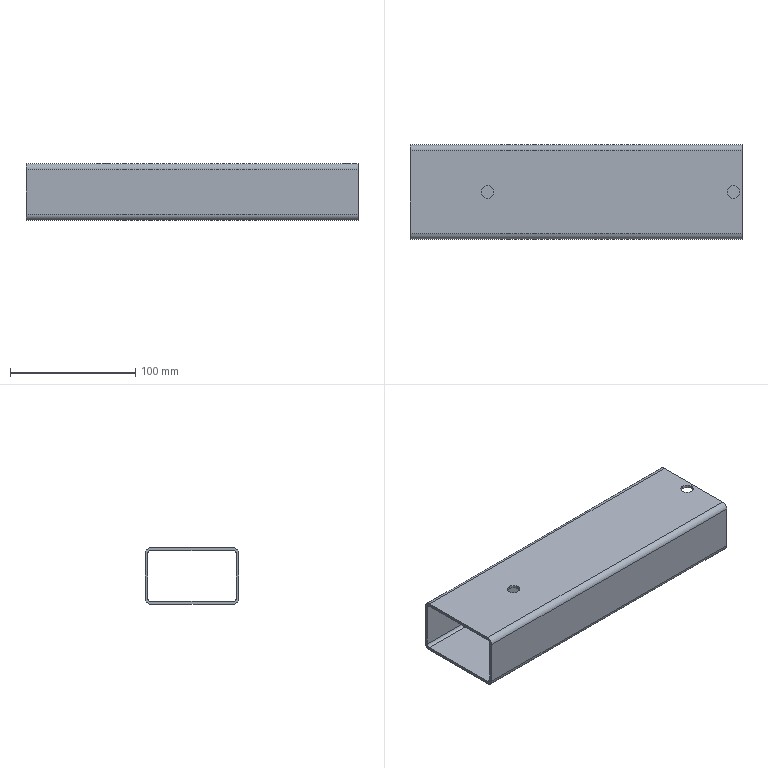Part | STEP file | [04]-1 | 1 solid | 22 faces | box 265 x 75 x 45 mm | volume 136701 mm3 | cylinder 12 | plane 10 | commonest cylinder face diameters 4.6 x4 9.2 x4 10 x4
STEP:
#1=CARTESIAN_POINT('',(81.9,42.5,45.));
#2=VERTEX_POINT('',#1);
#3=CARTESIAN_POINT('',(81.9,32.5,45.));
#4=VERTEX_POINT('',#3);
#5=CARTESIAN_POINT('',(81.9,37.5,45.));
#6=DIRECTION('',(0.,0.,-1.));
#7=DIRECTION('',(0.,-1.,0.));
#8=AXIS2_PLACEMENT_3D('',#5,#6,#7);
#9=CIRCLE('',#8,5.);
#10=EDGE_CURVE('',#2,#4,#9,.T.);
#11=ORIENTED_EDGE('',*,*,#10,.F.);
#12=CARTESIAN_POINT('',(81.9,42.5,42.7));
#13=VERTEX_POINT('',#12);
#14=CARTESIAN_POINT('',(81.9,42.5,45.));
#15=DIRECTION('',(0.,0.,-1.));
#16=VECTOR('',#15,1000.);
#17=LINE('',#14,#16);
#18=EDGE_CURVE('',#2,#13,#17,.T.);
#19=ORIENTED_EDGE('',*,*,#18,.T.);
#20=CARTESIAN_POINT('',(81.9,32.5,42.7));
#21=VERTEX_POINT('',#20);
#22=CARTESIAN_POINT('',(81.9,37.5,42.7));
#23=DIRECTION('',(0.,0.,1.));
#24=DIRECTION('',(0.,1.,0.));
#25=AXIS2_PLACEMENT_3D('',#22,#23,#24);
#26=CIRCLE('',#25,5.);
#27=EDGE_CURVE('',#21,#13,#26,.T.);
#28=ORIENTED_EDGE('',*,*,#27,.F.);
#29=CARTESIAN_POINT('',(81.9,32.5,45.));
#30=DIRECTION('',(0.,0.,-1.));
#31=VECTOR('',#30,1000.);
#32=LINE('',#29,#31);
#33=EDGE_CURVE('',#4,#21,#32,.T.);
#34=ORIENTED_EDGE('',*,*,#33,.F.);
#35=EDGE_LOOP('',(#11,#19,#28,#34));
#36=FACE_OUTER_BOUND('',#35,.T.);
#37=CARTESIAN_POINT('',(81.9,37.5,45.));
#38=DIRECTION('',(0.,0.,-1.));
#39=DIRECTION('',(0.,-1.,0.));
#40=AXIS2_PLACEMENT_3D('',#37,#38,#39);
#41=CYLINDRICAL_SURFACE('',#40,5.);
#42=ADVANCED_FACE('',(#36),#41,.F.);
#43=CARTESIAN_POINT('',(278.,42.5,45.));
#44=VERTEX_POINT('',#43);
#45=CARTESIAN_POINT('',(278.,32.5,45.));
#46=VERTEX_POINT('',#45);
#47=CARTESIAN_POINT('',(278.,37.5,45.));
#48=DIRECTION('',(0.,0.,-1.));
#49=DIRECTION('',(0.,-1.,0.));
#50=AXIS2_PLACEMENT_3D('',#47,#48,#49);
#51=CIRCLE('',#50,5.);
#52=EDGE_CURVE('',#44,#46,#51,.T.);
#53=ORIENTED_EDGE('',*,*,#52,.F.);
#54=CARTESIAN_POINT('',(278.,42.5,42.7));
#55=VERTEX_POINT('',#54);
#56=CARTESIAN_POINT('',(278.,42.5,45.));
#57=DIRECTION('',(0.,0.,-1.));
#58=VECTOR('',#57,1000.);
#59=LINE('',#56,#58);
#60=EDGE_CURVE('',#44,#55,#59,.T.);
#61=ORIENTED_EDGE('',*,*,#60,.T.);
#62=CARTESIAN_POINT('',(278.,32.5,42.7));
#63=VERTEX_POINT('',#62);
#64=CARTESIAN_POINT('',(278.,37.5,42.7));
#65=DIRECTION('',(0.,0.,1.));
#66=DIRECTION('',(0.,1.,0.));
#67=AXIS2_PLACEMENT_3D('',#64,#65,#66);
#68=CIRCLE('',#67,5.);
#69=EDGE_CURVE('',#63,#55,#68,.T.);
#70=ORIENTED_EDGE('',*,*,#69,.F.);
#71=CARTESIAN_POINT('',(278.,32.5,45.));
#72=DIRECTION('',(0.,0.,-1.));
#73=VECTOR('',#72,1000.);
#74=LINE('',#71,#73);
#75=EDGE_CURVE('',#46,#63,#74,.T.);
#76=ORIENTED_EDGE('',*,*,#75,.F.);
#77=EDGE_LOOP('',(#53,#61,#70,#76));
#78=FACE_OUTER_BOUND('',#77,.T.);
#79=CARTESIAN_POINT('',(278.,37.5,45.));
#80=DIRECTION('',(0.,0.,-1.));
#81=DIRECTION('',(0.,-1.,0.));
#82=AXIS2_PLACEMENT_3D('',#79,#80,#81);
#83=CYLINDRICAL_SURFACE('',#82,5.);
#84=ADVANCED_FACE('',(#78),#83,.F.);
#85=CARTESIAN_POINT('',(20.,70.4,0.));
#86=VERTEX_POINT('',#85);
#87=CARTESIAN_POINT('',(20.,4.6,0.));
#88=VERTEX_POINT('',#87);
#89=CARTESIAN_POINT('',(20.,70.4,0.));
#90=DIRECTION('',(0.,-1.,0.));
#91=VECTOR('',#90,1000.);
#92=LINE('',#89,#91);
#93=EDGE_CURVE('',#86,#88,#92,.T.);
#94=ORIENTED_EDGE('',*,*,#93,.T.);
#95=CARTESIAN_POINT('',(20.,0.,4.6));
#96=VERTEX_POINT('',#95);
#97=CARTESIAN_POINT('',(20.,4.6,4.6));
#98=DIRECTION('',(-1.,0.,0.));
#99=DIRECTION('',(0.,0.,-1.));
#100=AXIS2_PLACEMENT_3D('',#97,#98,#99);
#101=CIRCLE('',#100,4.6);
#102=EDGE_CURVE('',#88,#96,#101,.T.);
#103=ORIENTED_EDGE('',*,*,#102,.T.);
#104=CARTESIAN_POINT('',(20.,0.,40.4));
#105=VERTEX_POINT('',#104);
#106=CARTESIAN_POINT('',(20.,0.,4.6));
#107=DIRECTION('',(0.,0.,1.));
#108=VECTOR('',#107,1000.);
#109=LINE('',#106,#108);
#110=EDGE_CURVE('',#96,#105,#109,.T.);
#111=ORIENTED_EDGE('',*,*,#110,.T.);
#112=CARTESIAN_POINT('',(20.,4.6,45.));
#113=VERTEX_POINT('',#112);
#114=CARTESIAN_POINT('',(20.,4.6,40.4));
#115=DIRECTION('',(-1.,0.,0.));
#116=DIRECTION('',(0.,0.,-1.));
#117=AXIS2_PLACEMENT_3D('',#114,#115,#116);
#118=CIRCLE('',#117,4.6);
#119=EDGE_CURVE('',#105,#113,#118,.T.);
#120=ORIENTED_EDGE('',*,*,#119,.T.);
#121=CARTESIAN_POINT('',(20.,70.4,45.));
#122=VERTEX_POINT('',#121);
#123=CARTESIAN_POINT('',(20.,4.6,45.));
#124=DIRECTION('',(0.,1.,0.));
#125=VECTOR('',#124,1000.);
#126=LINE('',#123,#125);
#127=EDGE_CURVE('',#113,#122,#126,.T.);
#128=ORIENTED_EDGE('',*,*,#127,.T.);
#129=CARTESIAN_POINT('',(20.,75.,40.4));
#130=VERTEX_POINT('',#129);
#131=CARTESIAN_POINT('',(20.,70.4,40.4));
#132=DIRECTION('',(-1.,0.,0.));
#133=DIRECTION('',(0.,0.,-1.));
#134=AXIS2_PLACEMENT_3D('',#131,#132,#133);
#135=CIRCLE('',#134,4.6);
#136=EDGE_CURVE('',#122,#130,#135,.T.);
#137=ORIENTED_EDGE('',*,*,#136,.T.);
#138=CARTESIAN_POINT('',(20.,75.,4.6));
#139=VERTEX_POINT('',#138);
#140=CARTESIAN_POINT('',(20.,75.,40.4));
#141=DIRECTION('',(0.,0.,-1.));
#142=VECTOR('',#141,1000.);
#143=LINE('',#140,#142);
#144=EDGE_CURVE('',#130,#139,#143,.T.);
#145=ORIENTED_EDGE('',*,*,#144,.T.);
#146=CARTESIAN_POINT('',(20.,70.4,4.6));
#147=DIRECTION('',(-1.,0.,0.));
#148=DIRECTION('',(0.,0.,-1.));
#149=AXIS2_PLACEMENT_3D('',#146,#147,#148);
#150=CIRCLE('',#149,4.6);
#151=EDGE_CURVE('',#139,#86,#150,.T.);
#152=ORIENTED_EDGE('',*,*,#151,.T.);
#153=EDGE_LOOP('',(#94,#103,#111,#120,#128,#137,#145,#152));
#154=FACE_OUTER_BOUND('',#153,.T.);
#155=CARTESIAN_POINT('',(20.,70.4,2.3));
#156=VERTEX_POINT('',#155);
#157=CARTESIAN_POINT('',(20.,4.6,2.3));
#158=VERTEX_POINT('',#157);
#159=CARTESIAN_POINT('',(20.,70.4,2.3));
#160=DIRECTION('',(0.,-1.,0.));
#161=VECTOR('',#160,1000.);
#162=LINE('',#159,#161);
#163=EDGE_CURVE('',#156,#158,#162,.T.);
#164=ORIENTED_EDGE('',*,*,#163,.F.);
#165=CARTESIAN_POINT('',(20.,72.7,4.6));
#166=VERTEX_POINT('',#165);
#167=CARTESIAN_POINT('',(20.,70.4,4.6));
#168=DIRECTION('',(-1.,0.,0.));
#169=DIRECTION('',(0.,1.,0.));
#170=AXIS2_PLACEMENT_3D('',#167,#168,#169);
#171=CIRCLE('',#170,2.3);
#172=EDGE_CURVE('',#166,#156,#171,.T.);
#173=ORIENTED_EDGE('',*,*,#172,.F.);
#174=CARTESIAN_POINT('',(20.,72.7,40.4));
#175=VERTEX_POINT('',#174);
#176=CARTESIAN_POINT('',(20.,72.7,40.4));
#177=DIRECTION('',(0.,0.,-1.));
#178=VECTOR('',#177,1000.);
#179=LINE('',#176,#178);
#180=EDGE_CURVE('',#175,#166,#179,.T.);
#181=ORIENTED_EDGE('',*,*,#180,.F.);
#182=CARTESIAN_POINT('',(20.,70.4,42.7));
#183=VERTEX_POINT('',#182);
#184=CARTESIAN_POINT('',(20.,70.4,40.4));
#185=DIRECTION('',(-1.,0.,0.));
#186=DIRECTION('',(0.,1.,0.));
#187=AXIS2_PLACEMENT_3D('',#184,#185,#186);
#188=CIRCLE('',#187,2.3);
#189=EDGE_CURVE('',#183,#175,#188,.T.);
#190=ORIENTED_EDGE('',*,*,#189,.F.);
#191=CARTESIAN_POINT('',(20.,4.6,42.7));
#192=VERTEX_POINT('',#191);
#193=CARTESIAN_POINT('',(20.,4.6,42.7));
#194=DIRECTION('',(0.,1.,0.));
#195=VECTOR('',#194,1000.);
#196=LINE('',#193,#195);
#197=EDGE_CURVE('',#192,#183,#196,.T.);
#198=ORIENTED_EDGE('',*,*,#197,.F.);
#199=CARTESIAN_POINT('',(20.,2.3,40.4));
#200=VERTEX_POINT('',#199);
#201=CARTESIAN_POINT('',(20.,4.6,40.4));
#202=DIRECTION('',(-1.,0.,0.));
#203=DIRECTION('',(0.,1.,0.));
#204=AXIS2_PLACEMENT_3D('',#201,#202,#203);
#205=CIRCLE('',#204,2.3);
#206=EDGE_CURVE('',#200,#192,#205,.T.);
#207=ORIENTED_EDGE('',*,*,#206,.F.);
#208=CARTESIAN_POINT('',(20.,2.3,4.6));
#209=VERTEX_POINT('',#208);
#210=CARTESIAN_POINT('',(20.,2.3,4.6));
#211=DIRECTION('',(0.,0.,1.));
#212=VECTOR('',#211,1000.);
#213=LINE('',#210,#212);
#214=EDGE_CURVE('',#209,#200,#213,.T.);
#215=ORIENTED_EDGE('',*,*,#214,.F.);
#216=CARTESIAN_POINT('',(20.,4.6,4.6));
#217=DIRECTION('',(-1.,0.,0.));
#218=DIRECTION('',(0.,1.,0.));
#219=AXIS2_PLACEMENT_3D('',#216,#217,#218);
#220=CIRCLE('',#219,2.3);
#221=EDGE_CURVE('',#158,#209,#220,.T.);
#222=ORIENTED_EDGE('',*,*,#221,.F.);
#223=EDGE_LOOP('',(#164,#173,#181,#190,#198,#207,#215,#222));
#224=FACE_BOUND('',#223,.T.);
#225=CARTESIAN_POINT('',(20.,4.6,4.6));
#226=DIRECTION('',(-1.,0.,0.));
#227=DIRECTION('',(0.,0.,-1.));
#228=AXIS2_PLACEMENT_3D('',#225,#226,#227);
#229=PLANE('',#228);
#230=ADVANCED_FACE('',(#154,#224),#229,.T.);
#231=CARTESIAN_POINT('',(285.,70.4,0.));
#232=VERTEX_POINT('',#231);
#233=CARTESIAN_POINT('',(285.,4.6,0.));
#234=VERTEX_POINT('',#233);
#235=CARTESIAN_POINT('',(285.,70.4,0.));
#236=DIRECTION('',(0.,-1.,0.));
#237=VECTOR('',#236,1000.);
#238=LINE('',#235,#237);
#239=EDGE_CURVE('',#232,#234,#238,.T.);
#240=ORIENTED_EDGE('',*,*,#239,.F.);
#241=CARTESIAN_POINT('',(285.,75.,4.6));
#242=VERTEX_POINT('',#241);
#243=CARTESIAN_POINT('',(285.,70.4,4.6));
#244=DIRECTION('',(-1.,0.,0.));
#245=DIRECTION('',(0.,0.,-1.));
#246=AXIS2_PLACEMENT_3D('',#243,#244,#245);
#247=CIRCLE('',#246,4.6);
#248=EDGE_CURVE('',#242,#232,#247,.T.);
#249=ORIENTED_EDGE('',*,*,#248,.F.);
#250=CARTESIAN_POINT('',(285.,75.,40.4));
#251=VERTEX_POINT('',#250);
#252=CARTESIAN_POINT('',(285.,75.,40.4));
#253=DIRECTION('',(0.,0.,-1.));
#254=VECTOR('',#253,1000.);
#255=LINE('',#252,#254);
#256=EDGE_CURVE('',#251,#242,#255,.T.);
#257=ORIENTED_EDGE('',*,*,#256,.F.);
#258=CARTESIAN_POINT('',(285.,70.4,45.));
#259=VERTEX_POINT('',#258);
#260=CARTESIAN_POINT('',(285.,70.4,40.4));
#261=DIRECTION('',(-1.,0.,0.));
#262=DIRECTION('',(0.,0.,-1.));
#263=AXIS2_PLACEMENT_3D('',#260,#261,#262);
#264=CIRCLE('',#263,4.6);
#265=EDGE_CURVE('',#259,#251,#264,.T.);
#266=ORIENTED_EDGE('',*,*,#265,.F.);
#267=CARTESIAN_POINT('',(285.,4.6,45.));
#268=VERTEX_POINT('',#267);
#269=CARTESIAN_POINT('',(285.,4.6,45.));
#270=DIRECTION('',(0.,1.,0.));
#271=VECTOR('',#270,1000.);
#272=LINE('',#269,#271);
#273=EDGE_CURVE('',#268,#259,#272,.T.);
#274=ORIENTED_EDGE('',*,*,#273,.F.);
#275=CARTESIAN_POINT('',(285.,0.,40.4));
#276=VERTEX_POINT('',#275);
#277=CARTESIAN_POINT('',(285.,4.6,40.4));
#278=DIRECTION('',(-1.,0.,0.));
#279=DIRECTION('',(0.,0.,-1.));
#280=AXIS2_PLACEMENT_3D('',#277,#278,#279);
#281=CIRCLE('',#280,4.6);
#282=EDGE_CURVE('',#276,#268,#281,.T.);
#283=ORIENTED_EDGE('',*,*,#282,.F.);
#284=CARTESIAN_POINT('',(285.,0.,4.6));
#285=VERTEX_POINT('',#284);
#286=CARTESIAN_POINT('',(285.,0.,4.6));
#287=DIRECTION('',(0.,0.,1.));
#288=VECTOR('',#287,1000.);
#289=LINE('',#286,#288);
#290=EDGE_CURVE('',#285,#276,#289,.T.);
#291=ORIENTED_EDGE('',*,*,#290,.F.);
#292=CARTESIAN_POINT('',(285.,4.6,4.6));
#293=DIRECTION('',(-1.,0.,0.));
#294=DIRECTION('',(0.,0.,-1.));
#295=AXIS2_PLACEMENT_3D('',#292,#293,#294);
#296=CIRCLE('',#295,4.6);
#297=EDGE_CURVE('',#234,#285,#296,.T.);
#298=ORIENTED_EDGE('',*,*,#297,.F.);
#299=EDGE_LOOP('',(#240,#249,#257,#266,#274,#283,#291,#298));
#300=FACE_OUTER_BOUND('',#299,.T.);
#301=CARTESIAN_POINT('',(285.,72.7,4.6));
#302=VERTEX_POINT('',#301);
#303=CARTESIAN_POINT('',(285.,70.4,2.3));
#304=VERTEX_POINT('',#303);
#305=CARTESIAN_POINT('',(285.,70.4,4.6));
#306=DIRECTION('',(-1.,0.,0.));
#307=DIRECTION('',(0.,1.,0.));
#308=AXIS2_PLACEMENT_3D('',#305,#306,#307);
#309=CIRCLE('',#308,2.3);
#310=EDGE_CURVE('',#302,#304,#309,.T.);
#311=ORIENTED_EDGE('',*,*,#310,.T.);
#312=CARTESIAN_POINT('',(285.,4.6,2.3));
#313=VERTEX_POINT('',#312);
#314=CARTESIAN_POINT('',(285.,70.4,2.3));
#315=DIRECTION('',(0.,-1.,0.));
#316=VECTOR('',#315,1000.);
#317=LINE('',#314,#316);
#318=EDGE_CURVE('',#304,#313,#317,.T.);
#319=ORIENTED_EDGE('',*,*,#318,.T.);
#320=CARTESIAN_POINT('',(285.,2.3,4.6));
#321=VERTEX_POINT('',#320);
#322=CARTESIAN_POINT('',(285.,4.6,4.6));
#323=DIRECTION('',(-1.,0.,0.));
#324=DIRECTION('',(0.,1.,0.));
#325=AXIS2_PLACEMENT_3D('',#322,#323,#324);
#326=CIRCLE('',#325,2.3);
#327=EDGE_CURVE('',#313,#321,#326,.T.);
#328=ORIENTED_EDGE('',*,*,#327,.T.);
#329=CARTESIAN_POINT('',(285.,2.3,40.4));
#330=VERTEX_POINT('',#329);
#331=CARTESIAN_POINT('',(285.,2.3,4.6));
#332=DIRECTION('',(0.,0.,1.));
#333=VECTOR('',#332,1000.);
#334=LINE('',#331,#333);
#335=EDGE_CURVE('',#321,#330,#334,.T.);
#336=ORIENTED_EDGE('',*,*,#335,.T.);
#337=CARTESIAN_POINT('',(285.,4.6,42.7));
#338=VERTEX_POINT('',#337);
#339=CARTESIAN_POINT('',(285.,4.6,40.4));
#340=DIRECTION('',(-1.,0.,0.));
#341=DIRECTION('',(0.,1.,0.));
#342=AXIS2_PLACEMENT_3D('',#339,#340,#341);
#343=CIRCLE('',#342,2.3);
#344=EDGE_CURVE('',#330,#338,#343,.T.);
#345=ORIENTED_EDGE('',*,*,#344,.T.);
#346=CARTESIAN_POINT('',(285.,70.4,42.7));
#347=VERTEX_POINT('',#346);
#348=CARTESIAN_POINT('',(285.,4.6,42.7));
#349=DIRECTION('',(0.,1.,0.));
#350=VECTOR('',#349,1000.);
#351=LINE('',#348,#350);
#352=EDGE_CURVE('',#338,#347,#351,.T.);
#353=ORIENTED_EDGE('',*,*,#352,.T.);
#354=CARTESIAN_POINT('',(285.,72.7,40.4));
#355=VERTEX_POINT('',#354);
#356=CARTESIAN_POINT('',(285.,70.4,40.4));
#357=DIRECTION('',(-1.,0.,0.));
#358=DIRECTION('',(0.,1.,0.));
#359=AXIS2_PLACEMENT_3D('',#356,#357,#358);
#360=CIRCLE('',#359,2.3);
#361=EDGE_CURVE('',#347,#355,#360,.T.);
#362=ORIENTED_EDGE('',*,*,#361,.T.);
#363=CARTESIAN_POINT('',(285.,72.7,40.4));
#364=DIRECTION('',(0.,0.,-1.));
#365=VECTOR('',#364,1000.);
#366=LINE('',#363,#365);
#367=EDGE_CURVE('',#355,#302,#366,.T.);
#368=ORIENTED_EDGE('',*,*,#367,.T.);
#369=EDGE_LOOP('',(#311,#319,#328,#336,#345,#353,#362,#368));
#370=FACE_BOUND('',#369,.T.);
#371=CARTESIAN_POINT('',(285.,4.6,4.6));
#372=DIRECTION('',(-1.,0.,0.));
#373=DIRECTION('',(0.,0.,-1.));
#374=AXIS2_PLACEMENT_3D('',#371,#372,#373);
#375=PLANE('',#374);
#376=ADVANCED_FACE('',(#300,#370),#375,.F.);
#377=ORIENTED_EDGE('',*,*,#239,.T.);
#378=CARTESIAN_POINT('',(20.,4.6,0.));
#379=DIRECTION('',(1.,0.,0.));
#380=VECTOR('',#379,1000.);
#381=LINE('',#378,#380);
#382=EDGE_CURVE('',#88,#234,#381,.T.);
#383=ORIENTED_EDGE('',*,*,#382,.F.);
#384=ORIENTED_EDGE('',*,*,#93,.F.);
#385=CARTESIAN_POINT('',(20.,70.4,0.));
#386=DIRECTION('',(1.,0.,0.));
#387=VECTOR('',#386,1000.);
#388=LINE('',#385,#387);
#389=EDGE_CURVE('',#86,#232,#388,.T.);
#390=ORIENTED_EDGE('',*,*,#389,.T.);
#391=EDGE_LOOP('',(#377,#383,#384,#390));
#392=FACE_OUTER_BOUND('',#391,.T.);
#393=CARTESIAN_POINT('',(20.,70.4,0.));
#394=DIRECTION('',(0.,0.,1.));
#395=DIRECTION('',(0.,1.,0.));
#396=AXIS2_PLACEMENT_3D('',#393,#394,#395);
#397=PLANE('',#396);
#398=ADVANCED_FACE('',(#392),#397,.F.);
#399=ORIENTED_EDGE('',*,*,#297,.T.);
#400=CARTESIAN_POINT('',(20.,0.,4.6));
#401=DIRECTION('',(1.,0.,0.));
#402=VECTOR('',#401,1000.);
#403=LINE('',#400,#402);
#404=EDGE_CURVE('',#96,#285,#403,.T.);
#405=ORIENTED_EDGE('',*,*,#404,.F.);
#406=ORIENTED_EDGE('',*,*,#102,.F.);
#407=ORIENTED_EDGE('',*,*,#382,.T.);
#408=EDGE_LOOP('',(#399,#405,#406,#407));
#409=FACE_OUTER_BOUND('',#408,.T.);
#410=CARTESIAN_POINT('',(20.,4.6,4.6));
#411=DIRECTION('',(1.,0.,0.));
#412=DIRECTION('',(0.,0.,1.));
#413=AXIS2_PLACEMENT_3D('',#410,#411,#412);
#414=CYLINDRICAL_SURFACE('',#413,4.6);
#415=ADVANCED_FACE('',(#409),#414,.T.);
#416=ORIENTED_EDGE('',*,*,#290,.T.);
#417=CARTESIAN_POINT('',(20.,0.,40.4));
#418=DIRECTION('',(1.,0.,0.));
#419=VECTOR('',#418,1000.);
#420=LINE('',#417,#419);
#421=EDGE_CURVE('',#105,#276,#420,.T.);
#422=ORIENTED_EDGE('',*,*,#421,.F.);
#423=ORIENTED_EDGE('',*,*,#110,.F.);
#424=ORIENTED_EDGE('',*,*,#404,.T.);
#425=EDGE_LOOP('',(#416,#422,#423,#424));
#426=FACE_OUTER_BOUND('',#425,.T.);
#427=CARTESIAN_POINT('',(20.,0.,4.6));
#428=DIRECTION('',(0.,1.,0.));
#429=DIRECTION('',(0.,0.,-1.));
#430=AXIS2_PLACEMENT_3D('',#427,#428,#429);
#431=PLANE('',#430);
#432=ADVANCED_FACE('',(#426),#431,.F.);
#433=ORIENTED_EDGE('',*,*,#282,.T.);
#434=CARTESIAN_POINT('',(20.,4.6,45.));
#435=DIRECTION('',(1.,0.,0.));
#436=VECTOR('',#435,1000.);
#437=LINE('',#434,#436);
#438=EDGE_CURVE('',#113,#268,#437,.T.);
#439=ORIENTED_EDGE('',*,*,#438,.F.);
#440=ORIENTED_EDGE('',*,*,#119,.F.);
#441=ORIENTED_EDGE('',*,*,#421,.T.);
#442=EDGE_LOOP('',(#433,#439,#440,#441));
#443=FACE_OUTER_BOUND('',#442,.T.);
#444=CARTESIAN_POINT('',(20.,4.6,40.4));
#445=DIRECTION('',(1.,0.,0.));
#446=DIRECTION('',(0.,0.,1.));
#447=AXIS2_PLACEMENT_3D('',#444,#445,#446);
#448=CYLINDRICAL_SURFACE('',#447,4.6);
#449=ADVANCED_FACE('',(#443),#448,.T.);
#450=CARTESIAN_POINT('',(81.9,37.5,45.));
#451=DIRECTION('',(0.,0.,-1.));
#452=DIRECTION('',(0.,-1.,0.));
#453=AXIS2_PLACEMENT_3D('',#450,#451,#452);
#454=CIRCLE('',#453,5.);
#455=EDGE_CURVE('',#4,#2,#454,.T.);
#456=ORIENTED_EDGE('',*,*,#455,.T.);
#457=ORIENTED_EDGE('',*,*,#10,.T.);
#458=EDGE_LOOP('',(#456,#457));
#459=FACE_BOUND('',#458,.T.);
#460=CARTESIAN_POINT('',(278.,37.5,45.));
#461=DIRECTION('',(0.,0.,-1.));
#462=DIRECTION('',(0.,-1.,0.));
#463=AXIS2_PLACEMENT_3D('',#460,#461,#462);
#464=CIRCLE('',#463,5.);
#465=EDGE_CURVE('',#46,#44,#464,.T.);
#466=ORIENTED_EDGE('',*,*,#465,.T.);
#467=ORIENTED_EDGE('',*,*,#52,.T.);
#468=EDGE_LOOP('',(#466,#467));
#469=FACE_BOUND('',#468,.T.);
#470=ORIENTED_EDGE('',*,*,#273,.T.);
#471=CARTESIAN_POINT('',(20.,70.4,45.));
#472=DIRECTION('',(1.,0.,0.));
#473=VECTOR('',#472,1000.);
#474=LINE('',#471,#473);
#475=EDGE_CURVE('',#122,#259,#474,.T.);
#476=ORIENTED_EDGE('',*,*,#475,.F.);
#477=ORIENTED_EDGE('',*,*,#127,.F.);
#478=ORIENTED_EDGE('',*,*,#438,.T.);
#479=EDGE_LOOP('',(#470,#476,#477,#478));
#480=FACE_OUTER_BOUND('',#479,.T.);
#481=CARTESIAN_POINT('',(20.,4.6,45.));
#482=DIRECTION('',(0.,0.,-1.));
#483=DIRECTION('',(0.,-1.,0.));
#484=AXIS2_PLACEMENT_3D('',#481,#482,#483);
#485=PLANE('',#484);
#486=ADVANCED_FACE('',(#459,#469,#480),#485,.F.);
#487=ORIENTED_EDGE('',*,*,#265,.T.);
#488=CARTESIAN_POINT('',(20.,75.,40.4));
#489=DIRECTION('',(1.,0.,0.));
#490=VECTOR('',#489,1000.);
#491=LINE('',#488,#490);
#492=EDGE_CURVE('',#130,#251,#491,.T.);
#493=ORIENTED_EDGE('',*,*,#492,.F.);
#494=ORIENTED_EDGE('',*,*,#136,.F.);
#495=ORIENTED_EDGE('',*,*,#475,.T.);
#496=EDGE_LOOP('',(#487,#493,#494,#495));
#497=FACE_OUTER_BOUND('',#496,.T.);
#498=CARTESIAN_POINT('',(20.,70.4,40.4));
#499=DIRECTION('',(1.,0.,0.));
#500=DIRECTION('',(0.,0.,1.));
#501=AXIS2_PLACEMENT_3D('',#498,#499,#500);
#502=CYLINDRICAL_SURFACE('',#501,4.6);
#503=ADVANCED_FACE('',(#497),#502,.T.);
#504=ORIENTED_EDGE('',*,*,#256,.T.);
#505=CARTESIAN_POINT('',(20.,75.,4.6));
#506=DIRECTION('',(1.,0.,0.));
#507=VECTOR('',#506,1000.);
#508=LINE('',#505,#507);
#509=EDGE_CURVE('',#139,#242,#508,.T.);
#510=ORIENTED_EDGE('',*,*,#509,.F.);
#511=ORIENTED_EDGE('',*,*,#144,.F.);
#512=ORIENTED_EDGE('',*,*,#492,.T.);
#513=EDGE_LOOP('',(#504,#510,#511,#512));
#514=FACE_OUTER_BOUND('',#513,.T.);
#515=CARTESIAN_POINT('',(20.,75.,40.4));
#516=DIRECTION('',(0.,-1.,0.));
#517=DIRECTION('',(-1.,0.,0.));
#518=AXIS2_PLACEMENT_3D('',#515,#516,#517);
#519=PLANE('',#518);
#520=ADVANCED_FACE('',(#514),#519,.F.);
#521=ORIENTED_EDGE('',*,*,#248,.T.);
#522=ORIENTED_EDGE('',*,*,#389,.F.);
#523=ORIENTED_EDGE('',*,*,#151,.F.);
#524=ORIENTED_EDGE('',*,*,#509,.T.);
#525=EDGE_LOOP('',(#521,#522,#523,#524));
#526=FACE_OUTER_BOUND('',#525,.T.);
#527=CARTESIAN_POINT('',(20.,70.4,4.6));
#528=DIRECTION('',(1.,0.,0.));
#529=DIRECTION('',(0.,0.,1.));
#530=AXIS2_PLACEMENT_3D('',#527,#528,#529);
#531=CYLINDRICAL_SURFACE('',#530,4.6);
#532=ADVANCED_FACE('',(#526),#531,.T.);
#533=ORIENTED_EDGE('',*,*,#310,.F.);
#534=CARTESIAN_POINT('',(20.,72.7,4.6));
#535=DIRECTION('',(1.,0.,0.));
#536=VECTOR('',#535,1000.);
#537=LINE('',#534,#536);
#538=EDGE_CURVE('',#166,#302,#537,.T.);
#539=ORIENTED_EDGE('',*,*,#538,.F.);
#540=ORIENTED_EDGE('',*,*,#172,.T.);
#541=CARTESIAN_POINT('',(20.,70.4,2.3));
#542=DIRECTION('',(1.,0.,0.));
#543=VECTOR('',#542,1000.);
#544=LINE('',#541,#543);
#545=EDGE_CURVE('',#156,#304,#544,.T.);
#546=ORIENTED_EDGE('',*,*,#545,.T.);
#547=EDGE_LOOP('',(#533,#539,#540,#546));
#548=FACE_OUTER_BOUND('',#547,.T.);
#549=CARTESIAN_POINT('',(20.,70.4,4.6));
#550=DIRECTION('',(1.,0.,0.));
#551=DIRECTION('',(0.,-1.,0.));
#552=AXIS2_PLACEMENT_3D('',#549,#550,#551);
#553=CYLINDRICAL_SURFACE('',#552,2.3);
#554=ADVANCED_FACE('',(#548),#553,.F.);
#555=ORIENTED_EDGE('',*,*,#318,.F.);
#556=ORIENTED_EDGE('',*,*,#545,.F.);
#557=ORIENTED_EDGE('',*,*,#163,.T.);
#558=CARTESIAN_POINT('',(20.,4.6,2.3));
#559=DIRECTION('',(1.,0.,0.));
#560=VECTOR('',#559,1000.);
#561=LINE('',#558,#560);
#562=EDGE_CURVE('',#158,#313,#561,.T.);
#563=ORIENTED_EDGE('',*,*,#562,.T.);
#564=EDGE_LOOP('',(#555,#556,#557,#563));
#565=FACE_OUTER_BOUND('',#564,.T.);
#566=CARTESIAN_POINT('',(20.,70.4,2.3));
#567=DIRECTION('',(0.,0.,1.));
#568=DIRECTION('',(1.,0.,0.));
#569=AXIS2_PLACEMENT_3D('',#566,#567,#568);
#570=PLANE('',#569);
#571=ADVANCED_FACE('',(#565),#570,.T.);
#572=ORIENTED_EDGE('',*,*,#327,.F.);
#573=ORIENTED_EDGE('',*,*,#562,.F.);
#574=ORIENTED_EDGE('',*,*,#221,.T.);
#575=CARTESIAN_POINT('',(20.,2.3,4.6));
#576=DIRECTION('',(1.,0.,0.));
#577=VECTOR('',#576,1000.);
#578=LINE('',#575,#577);
#579=EDGE_CURVE('',#209,#321,#578,.T.);
#580=ORIENTED_EDGE('',*,*,#579,.T.);
#581=EDGE_LOOP('',(#572,#573,#574,#580));
#582=FACE_OUTER_BOUND('',#581,.T.);
#583=CARTESIAN_POINT('',(20.,4.6,4.6));
#584=DIRECTION('',(1.,0.,0.));
#585=DIRECTION('',(0.,-1.,0.));
#586=AXIS2_PLACEMENT_3D('',#583,#584,#585);
#587=CYLINDRICAL_SURFACE('',#586,2.3);
#588=ADVANCED_FACE('',(#582),#587,.F.);
#589=ORIENTED_EDGE('',*,*,#335,.F.);
#590=ORIENTED_EDGE('',*,*,#579,.F.);
#591=ORIENTED_EDGE('',*,*,#214,.T.);
#592=CARTESIAN_POINT('',(20.,2.3,40.4));
#593=DIRECTION('',(1.,0.,0.));
#594=VECTOR('',#593,1000.);
#595=LINE('',#592,#594);
#596=EDGE_CURVE('',#200,#330,#595,.T.);
#597=ORIENTED_EDGE('',*,*,#596,.T.);
#598=EDGE_LOOP('',(#589,#590,#591,#597));
#599=FACE_OUTER_BOUND('',#598,.T.);
#600=CARTESIAN_POINT('',(20.,2.3,4.6));
#601=DIRECTION('',(0.,1.,0.));
#602=DIRECTION('',(1.,0.,0.));
#603=AXIS2_PLACEMENT_3D('',#600,#601,#602);
#604=PLANE('',#603);
#605=ADVANCED_FACE('',(#599),#604,.T.);
#606=ORIENTED_EDGE('',*,*,#344,.F.);
#607=ORIENTED_EDGE('',*,*,#596,.F.);
#608=ORIENTED_EDGE('',*,*,#206,.T.);
#609=CARTESIAN_POINT('',(20.,4.6,42.7));
#610=DIRECTION('',(1.,0.,0.));
#611=VECTOR('',#610,1000.);
#612=LINE('',#609,#611);
#613=EDGE_CURVE('',#192,#338,#612,.T.);
#614=ORIENTED_EDGE('',*,*,#613,.T.);
#615=EDGE_LOOP('',(#606,#607,#608,#614));
#616=FACE_OUTER_BOUND('',#615,.T.);
#617=CARTESIAN_POINT('',(20.,4.6,40.4));
#618=DIRECTION('',(1.,0.,0.));
#619=DIRECTION('',(0.,-1.,0.));
#620=AXIS2_PLACEMENT_3D('',#617,#618,#619);
#621=CYLINDRICAL_SURFACE('',#620,2.3);
#622=ADVANCED_FACE('',(#616),#621,.F.);
#623=ORIENTED_EDGE('',*,*,#27,.T.);
#624=CARTESIAN_POINT('',(81.9,37.5,42.7));
#625=DIRECTION('',(0.,0.,1.));
#626=DIRECTION('',(0.,1.,0.));
#627=AXIS2_PLACEMENT_3D('',#624,#625,#626);
#628=CIRCLE('',#627,5.);
#629=EDGE_CURVE('',#13,#21,#628,.T.);
#630=ORIENTED_EDGE('',*,*,#629,.T.);
#631=EDGE_LOOP('',(#623,#630));
#632=FACE_BOUND('',#631,.T.);
#633=ORIENTED_EDGE('',*,*,#69,.T.);
#634=CARTESIAN_POINT('',(278.,37.5,42.7));
#635=DIRECTION('',(0.,0.,1.));
#636=DIRECTION('',(0.,1.,0.));
#637=AXIS2_PLACEMENT_3D('',#634,#635,#636);
#638=CIRCLE('',#637,5.);
#639=EDGE_CURVE('',#55,#63,#638,.T.);
#640=ORIENTED_EDGE('',*,*,#639,.T.);
#641=EDGE_LOOP('',(#633,#640));
#642=FACE_BOUND('',#641,.T.);
#643=ORIENTED_EDGE('',*,*,#352,.F.);
#644=ORIENTED_EDGE('',*,*,#613,.F.);
#645=ORIENTED_EDGE('',*,*,#197,.T.);
#646=CARTESIAN_POINT('',(20.,70.4,42.7));
#647=DIRECTION('',(1.,0.,0.));
#648=VECTOR('',#647,1000.);
#649=LINE('',#646,#648);
#650=EDGE_CURVE('',#183,#347,#649,.T.);
#651=ORIENTED_EDGE('',*,*,#650,.T.);
#652=EDGE_LOOP('',(#643,#644,#645,#651));
#653=FACE_OUTER_BOUND('',#652,.T.);
#654=CARTESIAN_POINT('',(20.,4.6,42.7));
#655=DIRECTION('',(0.,0.,-1.));
#656=DIRECTION('',(0.,-1.,0.));
#657=AXIS2_PLACEMENT_3D('',#654,#655,#656);
#658=PLANE('',#657);
#659=ADVANCED_FACE('',(#632,#642,#653),#658,.T.);
#660=ORIENTED_EDGE('',*,*,#361,.F.);
#661=ORIENTED_EDGE('',*,*,#650,.F.);
#662=ORIENTED_EDGE('',*,*,#189,.T.);
#663=CARTESIAN_POINT('',(20.,72.7,40.4));
#664=DIRECTION('',(1.,0.,0.));
#665=VECTOR('',#664,1000.);
#666=LINE('',#663,#665);
#667=EDGE_CURVE('',#175,#355,#666,.T.);
#668=ORIENTED_EDGE('',*,*,#667,.T.);
#669=EDGE_LOOP('',(#660,#661,#662,#668));
#670=FACE_OUTER_BOUND('',#669,.T.);
#671=CARTESIAN_POINT('',(20.,70.4,40.4));
#672=DIRECTION('',(1.,0.,0.));
#673=DIRECTION('',(0.,-1.,0.));
#674=AXIS2_PLACEMENT_3D('',#671,#672,#673);
#675=CYLINDRICAL_SURFACE('',#674,2.3);
#676=ADVANCED_FACE('',(#670),#675,.F.);
#677=ORIENTED_EDGE('',*,*,#367,.F.);
#678=ORIENTED_EDGE('',*,*,#667,.F.);
#679=ORIENTED_EDGE('',*,*,#180,.T.);
#680=ORIENTED_EDGE('',*,*,#538,.T.);
#681=EDGE_LOOP('',(#677,#678,#679,#680));
#682=FACE_OUTER_BOUND('',#681,.T.);
#683=CARTESIAN_POINT('',(20.,72.7,40.4));
#684=DIRECTION('',(0.,-1.,0.));
#685=DIRECTION('',(0.,0.,1.));
#686=AXIS2_PLACEMENT_3D('',#683,#684,#685);
#687=PLANE('',#686);
#688=ADVANCED_FACE('',(#682),#687,.T.);
#689=ORIENTED_EDGE('',*,*,#60,.F.);
#690=ORIENTED_EDGE('',*,*,#465,.F.);
#691=ORIENTED_EDGE('',*,*,#75,.T.);
#692=ORIENTED_EDGE('',*,*,#639,.F.);
#693=EDGE_LOOP('',(#689,#690,#691,#692));
#694=FACE_OUTER_BOUND('',#693,.T.);
#695=CARTESIAN_POINT('',(278.,37.5,45.));
#696=DIRECTION('',(0.,0.,-1.));
#697=DIRECTION('',(0.,-1.,0.));
#698=AXIS2_PLACEMENT_3D('',#695,#696,#697);
#699=CYLINDRICAL_SURFACE('',#698,5.);
#700=ADVANCED_FACE('',(#694),#699,.F.);
#701=ORIENTED_EDGE('',*,*,#18,.F.);
#702=ORIENTED_EDGE('',*,*,#455,.F.);
#703=ORIENTED_EDGE('',*,*,#33,.T.);
#704=ORIENTED_EDGE('',*,*,#629,.F.);
#705=EDGE_LOOP('',(#701,#702,#703,#704));
#706=FACE_OUTER_BOUND('',#705,.T.);
#707=CARTESIAN_POINT('',(81.9,37.5,45.));
#708=DIRECTION('',(0.,0.,-1.));
#709=DIRECTION('',(0.,-1.,0.));
#710=AXIS2_PLACEMENT_3D('',#707,#708,#709);
#711=CYLINDRICAL_SURFACE('',#710,5.);
#712=ADVANCED_FACE('',(#706),#711,.F.);
#713=CLOSED_SHELL('',(#42,#84,#230,#376,#398,#415,#432,#449,#486,#503,#520,#532,#554,#571,#588,#605,#622,#659,#676,#688,#700,#712));
#714=MANIFOLD_SOLID_BREP('',#713);
#715=CARTESIAN_POINT('',(0.,0.,0.));
#716=DIRECTION('',(0.,0.,1.));
#717=DIRECTION('',(1.,0.,0.));
#718=AXIS2_PLACEMENT_3D('',#715,#716,#717);
#719=(LENGTH_UNIT()NAMED_UNIT(*)SI_UNIT(.MILLI.,.METRE.));
#720=UNCERTAINTY_MEASURE_WITH_UNIT(LENGTH_MEASURE(0.00001),#719,'','');
#721=(NAMED_UNIT(*)PLANE_ANGLE_UNIT()SI_UNIT($,.RADIAN.));
#722=(NAMED_UNIT(*)SI_UNIT($,.STERADIAN.)SOLID_ANGLE_UNIT());
#723=(GEOMETRIC_REPRESENTATION_CONTEXT(3)GLOBAL_UNCERTAINTY_ASSIGNED_CONTEXT((#720))GLOBAL_UNIT_ASSIGNED_CONTEXT((#719,#721,#722))REPRESENTATION_CONTEXT('',''));
#724=ADVANCED_BREP_SHAPE_REPRESENTATION('',(#714,#718),#723);